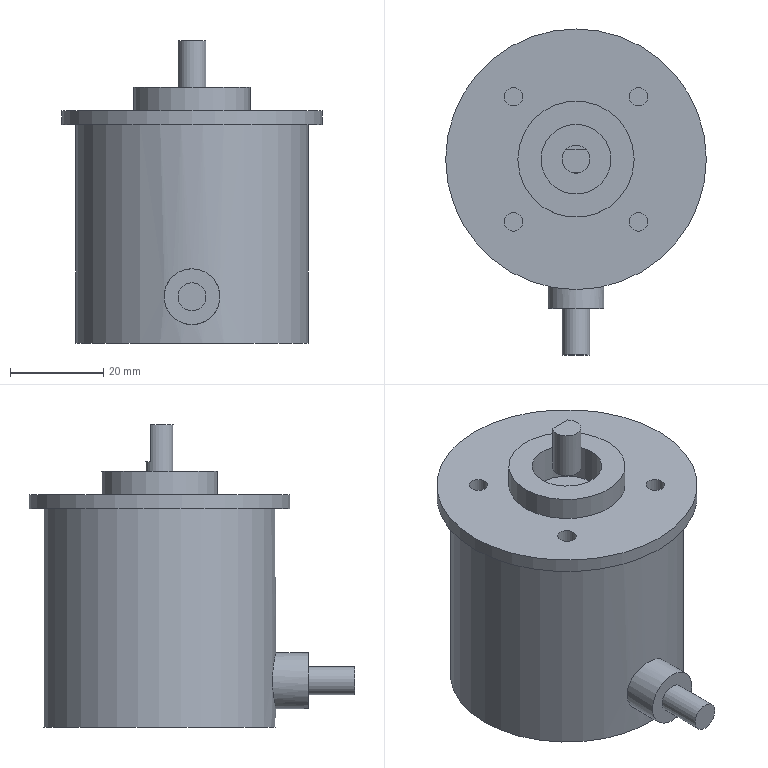Part | NX | features BREP 2 | 2 solids | 26 faces | box 56 x 70 x 65 mm | volume 101579 mm3 | plane 15 | cylinder 11 | commonest cylinder face diameters 4 x4 6 x2 12 x1 15 x1 25 x1 50 x1
STEP:
#1=CARTESIAN_POINT('',(-10.435,-13.435,4.5));
#2=VERTEX_POINT('',#1);
#3=CARTESIAN_POINT('',(-13.435,-13.435,4.5));
#4=DIRECTION('',(0.,0.,-1.));
#5=DIRECTION('',(1.,0.,0.));
#6=AXIS2_PLACEMENT_3D('',#3,#4,#5);
#7=CIRCLE('',#6,3.);
#8=EDGE_CURVE('',#2,#2,#7,.T.);
#9=ORIENTED_EDGE('',*,*,#8,.F.);
#10=EDGE_LOOP('',(#9));
#11=FACE_BOUND('',#10,.T.);
#12=CARTESIAN_POINT('',(-11.199,-11.435,15.));
#13=VERTEX_POINT('',#12);
#14=CARTESIAN_POINT('',(-15.671,-11.435,15.));
#15=VERTEX_POINT('',#14);
#16=CARTESIAN_POINT('',(-13.435,-13.435,15.));
#17=DIRECTION('',(0.,0.,-1.));
#18=DIRECTION('',(1.,0.,0.));
#19=AXIS2_PLACEMENT_3D('',#16,#17,#18);
#20=CIRCLE('',#19,3.);
#21=EDGE_CURVE('',#13,#15,#20,.T.);
#22=ORIENTED_EDGE('',*,*,#21,.T.);
#23=CARTESIAN_POINT('',(-15.671,-11.435,7.));
#24=VERTEX_POINT('',#23);
#25=CARTESIAN_POINT('',(-15.671,-11.435,7.));
#26=DIRECTION('',(0.,0.,-1.));
#27=VECTOR('',#26,1000.);
#28=LINE('',#25,#27);
#29=EDGE_CURVE('',#15,#24,#28,.T.);
#30=ORIENTED_EDGE('',*,*,#29,.T.);
#31=CARTESIAN_POINT('',(-11.199,-11.435,7.));
#32=VERTEX_POINT('',#31);
#33=CARTESIAN_POINT('',(-13.435,-13.435,7.));
#34=DIRECTION('',(0.,0.,1.));
#35=DIRECTION('',(1.,0.,0.));
#36=AXIS2_PLACEMENT_3D('',#33,#34,#35);
#37=CIRCLE('',#36,3.);
#38=EDGE_CURVE('',#32,#24,#37,.T.);
#39=ORIENTED_EDGE('',*,*,#38,.F.);
#40=CARTESIAN_POINT('',(-11.199,-11.435,7.));
#41=DIRECTION('',(0.,0.,-1.));
#42=VECTOR('',#41,1000.);
#43=LINE('',#40,#42);
#44=EDGE_CURVE('',#13,#32,#43,.T.);
#45=ORIENTED_EDGE('',*,*,#44,.F.);
#46=EDGE_LOOP('',(#22,#30,#39,#45));
#47=FACE_BOUND('',#46,.T.);
#48=CARTESIAN_POINT('',(-13.435,-13.435,15.));
#49=DIRECTION('',(0.,0.,-1.));
#50=DIRECTION('',(-1.,0.,0.));
#51=AXIS2_PLACEMENT_3D('',#48,#49,#50);
#52=CYLINDRICAL_SURFACE('',#51,3.);
#53=ADVANCED_FACE('',(#11,#47),#52,.T.);
#54=CARTESIAN_POINT('',(-15.671,-11.435,15.));
#55=DIRECTION('',(1.,0.,0.));
#56=VECTOR('',#55,1000.);
#57=LINE('',#54,#56);
#58=EDGE_CURVE('',#15,#13,#57,.T.);
#59=ORIENTED_EDGE('',*,*,#58,.F.);
#60=ORIENTED_EDGE('',*,*,#21,.F.);
#61=EDGE_LOOP('',(#59,#60));
#62=FACE_BOUND('',#61,.T.);
#63=CARTESIAN_POINT('',(-13.435,-13.435,15.));
#64=DIRECTION('',(0.,0.,1.));
#65=DIRECTION('',(1.,0.,0.));
#66=AXIS2_PLACEMENT_3D('',#63,#64,#65);
#67=PLANE('',#66);
#68=ADVANCED_FACE('',(#62),#67,.T.);
#69=ORIENTED_EDGE('',*,*,#8,.T.);
#70=EDGE_LOOP('',(#69));
#71=FACE_BOUND('',#70,.T.);
#72=CARTESIAN_POINT('',(-13.435,-13.435,4.5));
#73=DIRECTION('',(0.,0.,1.));
#74=DIRECTION('',(1.,0.,0.));
#75=AXIS2_PLACEMENT_3D('',#72,#73,#74);
#76=PLANE('',#75);
#77=ADVANCED_FACE('',(#71),#76,.F.);
#78=ORIENTED_EDGE('',*,*,#58,.T.);
#79=ORIENTED_EDGE('',*,*,#44,.T.);
#80=CARTESIAN_POINT('',(-15.671,-11.435,7.));
#81=DIRECTION('',(1.,0.,0.));
#82=VECTOR('',#81,1000.);
#83=LINE('',#80,#82);
#84=EDGE_CURVE('',#24,#32,#83,.T.);
#85=ORIENTED_EDGE('',*,*,#84,.F.);
#86=ORIENTED_EDGE('',*,*,#29,.F.);
#87=EDGE_LOOP('',(#78,#79,#85,#86));
#88=FACE_BOUND('',#87,.T.);
#89=CARTESIAN_POINT('',(-15.671,-11.435,7.));
#90=DIRECTION('',(0.,-1.,0.));
#91=DIRECTION('',(0.,0.,-1.));
#92=AXIS2_PLACEMENT_3D('',#89,#90,#91);
#93=PLANE('',#92);
#94=ADVANCED_FACE('',(#88),#93,.F.);
#95=ORIENTED_EDGE('',*,*,#38,.T.);
#96=ORIENTED_EDGE('',*,*,#84,.T.);
#97=EDGE_LOOP('',(#95,#96));
#98=FACE_BOUND('',#97,.T.);
#99=CARTESIAN_POINT('',(-13.435,-13.435,7.));
#100=DIRECTION('',(0.,0.,1.));
#101=DIRECTION('',(1.,0.,0.));
#102=AXIS2_PLACEMENT_3D('',#99,#100,#101);
#103=PLANE('',#102);
#104=ADVANCED_FACE('',(#98),#103,.T.);
#105=CLOSED_SHELL('',(#53,#68,#77,#94,#104));
#106=MANIFOLD_SOLID_BREP('',#105);
#107=CARTESIAN_POINT('',(2.,0.,0.));
#108=VERTEX_POINT('',#107);
#109=CARTESIAN_POINT('',(0.,0.,0.));
#110=DIRECTION('',(0.,0.,1.));
#111=DIRECTION('',(1.,0.,0.));
#112=AXIS2_PLACEMENT_3D('',#109,#110,#111);
#113=CIRCLE('',#112,2.);
#114=EDGE_CURVE('',#108,#108,#113,.T.);
#115=ORIENTED_EDGE('',*,*,#114,.T.);
#116=EDGE_LOOP('',(#115));
#117=FACE_BOUND('',#116,.T.);
#118=CARTESIAN_POINT('',(2.,0.,-10.));
#119=VERTEX_POINT('',#118);
#120=CARTESIAN_POINT('',(0.,0.,-10.));
#121=DIRECTION('',(0.,0.,1.));
#122=DIRECTION('',(1.,0.,0.));
#123=AXIS2_PLACEMENT_3D('',#120,#121,#122);
#124=CIRCLE('',#123,2.);
#125=EDGE_CURVE('',#119,#119,#124,.T.);
#126=ORIENTED_EDGE('',*,*,#125,.F.);
#127=EDGE_LOOP('',(#126));
#128=FACE_BOUND('',#127,.T.);
#129=CARTESIAN_POINT('',(0.,0.,0.));
#130=DIRECTION('',(0.,0.,1.));
#131=DIRECTION('',(1.,0.,0.));
#132=AXIS2_PLACEMENT_3D('',#129,#130,#131);
#133=CYLINDRICAL_SURFACE('',#132,2.);
#134=ADVANCED_FACE('',(#117,#128),#133,.F.);
#135=CARTESIAN_POINT('',(-24.87,0.,0.));
#136=VERTEX_POINT('',#135);
#137=CARTESIAN_POINT('',(-26.87,0.,0.));
#138=DIRECTION('',(0.,0.,1.));
#139=DIRECTION('',(1.,0.,0.));
#140=AXIS2_PLACEMENT_3D('',#137,#138,#139);
#141=CIRCLE('',#140,2.);
#142=EDGE_CURVE('',#136,#136,#141,.T.);
#143=ORIENTED_EDGE('',*,*,#142,.T.);
#144=EDGE_LOOP('',(#143));
#145=FACE_BOUND('',#144,.T.);
#146=CARTESIAN_POINT('',(-24.87,0.,-10.));
#147=VERTEX_POINT('',#146);
#148=CARTESIAN_POINT('',(-26.87,0.,-10.));
#149=DIRECTION('',(0.,0.,1.));
#150=DIRECTION('',(1.,0.,0.));
#151=AXIS2_PLACEMENT_3D('',#148,#149,#150);
#152=CIRCLE('',#151,2.);
#153=EDGE_CURVE('',#147,#147,#152,.T.);
#154=ORIENTED_EDGE('',*,*,#153,.F.);
#155=EDGE_LOOP('',(#154));
#156=FACE_BOUND('',#155,.T.);
#157=CARTESIAN_POINT('',(-26.87,0.,0.));
#158=DIRECTION('',(0.,0.,1.));
#159=DIRECTION('',(1.,0.,0.));
#160=AXIS2_PLACEMENT_3D('',#157,#158,#159);
#161=CYLINDRICAL_SURFACE('',#160,2.);
#162=ADVANCED_FACE('',(#145,#156),#161,.F.);
#163=CARTESIAN_POINT('',(-24.87,-26.87,0.));
#164=VERTEX_POINT('',#163);
#165=CARTESIAN_POINT('',(-26.87,-26.87,0.));
#166=DIRECTION('',(0.,0.,1.));
#167=DIRECTION('',(1.,0.,0.));
#168=AXIS2_PLACEMENT_3D('',#165,#166,#167);
#169=CIRCLE('',#168,2.);
#170=EDGE_CURVE('',#164,#164,#169,.T.);
#171=ORIENTED_EDGE('',*,*,#170,.T.);
#172=EDGE_LOOP('',(#171));
#173=FACE_BOUND('',#172,.T.);
#174=CARTESIAN_POINT('',(-24.87,-26.87,-10.));
#175=VERTEX_POINT('',#174);
#176=CARTESIAN_POINT('',(-26.87,-26.87,-10.));
#177=DIRECTION('',(0.,0.,1.));
#178=DIRECTION('',(1.,0.,0.));
#179=AXIS2_PLACEMENT_3D('',#176,#177,#178);
#180=CIRCLE('',#179,2.);
#181=EDGE_CURVE('',#175,#175,#180,.T.);
#182=ORIENTED_EDGE('',*,*,#181,.F.);
#183=EDGE_LOOP('',(#182));
#184=FACE_BOUND('',#183,.T.);
#185=CARTESIAN_POINT('',(-26.87,-26.87,0.));
#186=DIRECTION('',(0.,0.,1.));
#187=DIRECTION('',(1.,0.,0.));
#188=AXIS2_PLACEMENT_3D('',#185,#186,#187);
#189=CYLINDRICAL_SURFACE('',#188,2.);
#190=ADVANCED_FACE('',(#173,#184),#189,.F.);
#191=CARTESIAN_POINT('',(2.,-26.87,0.));
#192=VERTEX_POINT('',#191);
#193=CARTESIAN_POINT('',(0.,-26.87,0.));
#194=DIRECTION('',(0.,0.,1.));
#195=DIRECTION('',(1.,0.,0.));
#196=AXIS2_PLACEMENT_3D('',#193,#194,#195);
#197=CIRCLE('',#196,2.);
#198=EDGE_CURVE('',#192,#192,#197,.T.);
#199=ORIENTED_EDGE('',*,*,#198,.T.);
#200=EDGE_LOOP('',(#199));
#201=FACE_BOUND('',#200,.T.);
#202=CARTESIAN_POINT('',(2.,-26.87,-10.));
#203=VERTEX_POINT('',#202);
#204=CARTESIAN_POINT('',(0.,-26.87,-10.));
#205=DIRECTION('',(0.,0.,1.));
#206=DIRECTION('',(1.,0.,0.));
#207=AXIS2_PLACEMENT_3D('',#204,#205,#206);
#208=CIRCLE('',#207,2.);
#209=EDGE_CURVE('',#203,#203,#208,.T.);
#210=ORIENTED_EDGE('',*,*,#209,.F.);
#211=EDGE_LOOP('',(#210));
#212=FACE_BOUND('',#211,.T.);
#213=CARTESIAN_POINT('',(0.,-26.87,0.));
#214=DIRECTION('',(0.,0.,1.));
#215=DIRECTION('',(1.,0.,0.));
#216=AXIS2_PLACEMENT_3D('',#213,#214,#215);
#217=CYLINDRICAL_SURFACE('',#216,2.);
#218=ADVANCED_FACE('',(#201,#212),#217,.F.);
#219=CARTESIAN_POINT('',(-13.435,-55.435,-43.));
#220=VERTEX_POINT('',#219);
#221=CARTESIAN_POINT('',(-13.435,-55.435,-40.));
#222=DIRECTION('',(0.,-1.,0.));
#223=DIRECTION('',(0.,0.,-1.));
#224=AXIS2_PLACEMENT_3D('',#221,#222,#223);
#225=CIRCLE('',#224,3.);
#226=EDGE_CURVE('',#220,#220,#225,.T.);
#227=ORIENTED_EDGE('',*,*,#226,.F.);
#228=EDGE_LOOP('',(#227));
#229=FACE_BOUND('',#228,.T.);
#230=CARTESIAN_POINT('',(-13.435,-45.435,-43.));
#231=VERTEX_POINT('',#230);
#232=CARTESIAN_POINT('',(-13.435,-45.435,-40.));
#233=DIRECTION('',(0.,-1.,0.));
#234=DIRECTION('',(0.,0.,-1.));
#235=AXIS2_PLACEMENT_3D('',#232,#233,#234);
#236=CIRCLE('',#235,3.);
#237=EDGE_CURVE('',#231,#231,#236,.T.);
#238=ORIENTED_EDGE('',*,*,#237,.T.);
#239=EDGE_LOOP('',(#238));
#240=FACE_BOUND('',#239,.T.);
#241=CARTESIAN_POINT('',(-13.435,-37.704,-40.));
#242=DIRECTION('',(0.,-1.,0.));
#243=DIRECTION('',(0.,0.,-1.));
#244=AXIS2_PLACEMENT_3D('',#241,#242,#243);
#245=CYLINDRICAL_SURFACE('',#244,3.);
#246=ADVANCED_FACE('',(#229,#240),#245,.T.);
#247=CARTESIAN_POINT('',(-13.435,-45.435,-46.));
#248=VERTEX_POINT('',#247);
#249=CARTESIAN_POINT('',(-13.435,-45.435,-40.));
#250=DIRECTION('',(0.,-1.,0.));
#251=DIRECTION('',(0.,0.,-1.));
#252=AXIS2_PLACEMENT_3D('',#249,#250,#251);
#253=CIRCLE('',#252,6.);
#254=EDGE_CURVE('',#248,#248,#253,.T.);
#255=ORIENTED_EDGE('',*,*,#254,.F.);
#256=EDGE_LOOP('',(#255));
#257=FACE_BOUND('',#256,.T.);
#258=CARTESIAN_POINT('',(-13.435,-38.435,-34.));
#259=VERTEX_POINT('',#258);
#260=CARTESIAN_POINT('',(-18.141,-38.074,-35.302));
#261=CARTESIAN_POINT('',(-13.434,-38.615,-33.349));
#262=CARTESIAN_POINT('',(-8.732,-38.075,-35.302));
#263=CARTESIAN_POINT('',(-6.786,-37.519,-39.993));
#264=CARTESIAN_POINT('',(-8.733,-38.075,-44.703));
#265=CARTESIAN_POINT('',(-13.432,-38.615,-46.648));
#266=CARTESIAN_POINT('',(-18.133,-38.076,-44.706));
#267=CARTESIAN_POINT('',(-20.084,-37.519,-40.003));
#268=CARTESIAN_POINT('',(-18.141,-38.074,-35.302));
#269=CARTESIAN_POINT('',(-13.434,-38.615,-33.349));
#270=CARTESIAN_POINT('',(-8.732,-38.075,-35.302));
#271=B_SPLINE_CURVE_WITH_KNOTS('',3,(#260,#261,#262,#263,#264,#265,#266,#267,#268,#269,#270),.UNSPECIFIED.,.T.,.F.,(1,1,1,1,1,1,1,1,1,1,1,1,1,1,1),(-0.01412,-0.009413,-0.004706,0.,0.004706,0.009413,0.01412,0.01883,0.02353,0.02824,0.03294,0.03765,0.04236,0.04706,0.05177),.UNSPECIFIED.);
#272=EDGE_CURVE('',#259,#259,#271,.T.);
#273=ORIENTED_EDGE('',*,*,#272,.F.);
#274=EDGE_LOOP('',(#273));
#275=FACE_BOUND('',#274,.T.);
#276=CARTESIAN_POINT('',(-13.435,-37.704,-40.));
#277=DIRECTION('',(0.,-1.,0.));
#278=DIRECTION('',(0.,0.,-1.));
#279=AXIS2_PLACEMENT_3D('',#276,#277,#278);
#280=CYLINDRICAL_SURFACE('',#279,6.);
#281=ADVANCED_FACE('',(#257,#275),#280,.T.);
#282=CARTESIAN_POINT('',(-38.435,-13.435,-3.));
#283=VERTEX_POINT('',#282);
#284=CARTESIAN_POINT('',(-13.435,-13.435,-3.));
#285=DIRECTION('',(0.,0.,-1.));
#286=DIRECTION('',(-1.,0.,0.));
#287=AXIS2_PLACEMENT_3D('',#284,#285,#286);
#288=CIRCLE('',#287,25.);
#289=EDGE_CURVE('',#283,#283,#288,.T.);
#290=ORIENTED_EDGE('',*,*,#289,.T.);
#291=EDGE_LOOP('',(#290));
#292=FACE_BOUND('',#291,.T.);
#293=CARTESIAN_POINT('',(-38.435,-13.435,-50.));
#294=VERTEX_POINT('',#293);
#295=CARTESIAN_POINT('',(-13.435,-13.435,-50.));
#296=DIRECTION('',(0.,0.,-1.));
#297=DIRECTION('',(-1.,0.,0.));
#298=AXIS2_PLACEMENT_3D('',#295,#296,#297);
#299=CIRCLE('',#298,25.);
#300=EDGE_CURVE('',#294,#294,#299,.T.);
#301=ORIENTED_EDGE('',*,*,#300,.F.);
#302=EDGE_LOOP('',(#301));
#303=FACE_BOUND('',#302,.T.);
#304=ORIENTED_EDGE('',*,*,#272,.T.);
#305=EDGE_LOOP('',(#304));
#306=FACE_BOUND('',#305,.T.);
#307=CARTESIAN_POINT('',(-13.435,-13.435,-50.));
#308=DIRECTION('',(0.,0.,1.));
#309=DIRECTION('',(1.,0.,0.));
#310=AXIS2_PLACEMENT_3D('',#307,#308,#309);
#311=CYLINDRICAL_SURFACE('',#310,25.);
#312=ADVANCED_FACE('',(#292,#303,#306),#311,.T.);
#313=CARTESIAN_POINT('',(-5.935,-13.435,5.));
#314=VERTEX_POINT('',#313);
#315=CARTESIAN_POINT('',(-13.435,-13.435,5.));
#316=DIRECTION('',(0.,0.,1.));
#317=DIRECTION('',(1.,0.,0.));
#318=AXIS2_PLACEMENT_3D('',#315,#316,#317);
#319=CIRCLE('',#318,7.5);
#320=EDGE_CURVE('',#314,#314,#319,.T.);
#321=ORIENTED_EDGE('',*,*,#320,.T.);
#322=EDGE_LOOP('',(#321));
#323=FACE_BOUND('',#322,.T.);
#324=CARTESIAN_POINT('',(-5.935,-13.435,-3.));
#325=VERTEX_POINT('',#324);
#326=CARTESIAN_POINT('',(-13.435,-13.435,-3.));
#327=DIRECTION('',(0.,0.,1.));
#328=DIRECTION('',(1.,0.,0.));
#329=AXIS2_PLACEMENT_3D('',#326,#327,#328);
#330=CIRCLE('',#329,7.5);
#331=EDGE_CURVE('',#325,#325,#330,.T.);
#332=ORIENTED_EDGE('',*,*,#331,.F.);
#333=EDGE_LOOP('',(#332));
#334=FACE_BOUND('',#333,.T.);
#335=CARTESIAN_POINT('',(-13.435,-13.435,5.));
#336=DIRECTION('',(0.,0.,1.));
#337=DIRECTION('',(1.,0.,0.));
#338=AXIS2_PLACEMENT_3D('',#335,#336,#337);
#339=CYLINDRICAL_SURFACE('',#338,7.5);
#340=ADVANCED_FACE('',(#323,#334),#339,.F.);
#341=CARTESIAN_POINT('',(-0.935,-13.435,0.));
#342=VERTEX_POINT('',#341);
#343=CARTESIAN_POINT('',(-13.435,-13.435,0.));
#344=DIRECTION('',(0.,0.,1.));
#345=DIRECTION('',(1.,0.,0.));
#346=AXIS2_PLACEMENT_3D('',#343,#344,#345);
#347=CIRCLE('',#346,12.5);
#348=EDGE_CURVE('',#342,#342,#347,.T.);
#349=ORIENTED_EDGE('',*,*,#348,.T.);
#350=EDGE_LOOP('',(#349));
#351=FACE_BOUND('',#350,.T.);
#352=CARTESIAN_POINT('',(-0.935,-13.435,5.));
#353=VERTEX_POINT('',#352);
#354=CARTESIAN_POINT('',(-13.435,-13.435,5.));
#355=DIRECTION('',(0.,0.,1.));
#356=DIRECTION('',(1.,0.,0.));
#357=AXIS2_PLACEMENT_3D('',#354,#355,#356);
#358=CIRCLE('',#357,12.5);
#359=EDGE_CURVE('',#353,#353,#358,.T.);
#360=ORIENTED_EDGE('',*,*,#359,.F.);
#361=EDGE_LOOP('',(#360));
#362=FACE_BOUND('',#361,.T.);
#363=CARTESIAN_POINT('',(-13.435,-13.435,5.));
#364=DIRECTION('',(0.,0.,-1.));
#365=DIRECTION('',(-1.,0.,0.));
#366=AXIS2_PLACEMENT_3D('',#363,#364,#365);
#367=CYLINDRICAL_SURFACE('',#366,12.5);
#368=ADVANCED_FACE('',(#351,#362),#367,.T.);
#369=CARTESIAN_POINT('',(14.565,-13.435,0.));
#370=VERTEX_POINT('',#369);
#371=CARTESIAN_POINT('',(-13.435,-13.435,0.));
#372=DIRECTION('',(0.,0.,1.));
#373=DIRECTION('',(1.,0.,0.));
#374=AXIS2_PLACEMENT_3D('',#371,#372,#373);
#375=CIRCLE('',#374,28.);
#376=EDGE_CURVE('',#370,#370,#375,.T.);
#377=ORIENTED_EDGE('',*,*,#376,.F.);
#378=EDGE_LOOP('',(#377));
#379=FACE_BOUND('',#378,.T.);
#380=CARTESIAN_POINT('',(14.565,-13.435,-3.));
#381=VERTEX_POINT('',#380);
#382=CARTESIAN_POINT('',(-13.435,-13.435,-3.));
#383=DIRECTION('',(0.,0.,1.));
#384=DIRECTION('',(1.,0.,0.));
#385=AXIS2_PLACEMENT_3D('',#382,#383,#384);
#386=CIRCLE('',#385,28.);
#387=EDGE_CURVE('',#381,#381,#386,.T.);
#388=ORIENTED_EDGE('',*,*,#387,.T.);
#389=EDGE_LOOP('',(#388));
#390=FACE_BOUND('',#389,.T.);
#391=CARTESIAN_POINT('',(-13.435,-13.435,-3.));
#392=DIRECTION('',(0.,0.,1.));
#393=DIRECTION('',(1.,0.,0.));
#394=AXIS2_PLACEMENT_3D('',#391,#392,#393);
#395=CYLINDRICAL_SURFACE('',#394,28.);
#396=ADVANCED_FACE('',(#379,#390),#395,.T.);
#397=ORIENTED_EDGE('',*,*,#387,.F.);
#398=EDGE_LOOP('',(#397));
#399=FACE_BOUND('',#398,.T.);
#400=ORIENTED_EDGE('',*,*,#289,.F.);
#401=EDGE_LOOP('',(#400));
#402=FACE_BOUND('',#401,.T.);
#403=CARTESIAN_POINT('',(14.565,-13.435,-3.));
#404=DIRECTION('',(0.,0.,-1.));
#405=DIRECTION('',(-1.,0.,0.));
#406=AXIS2_PLACEMENT_3D('',#403,#404,#405);
#407=PLANE('',#406);
#408=ADVANCED_FACE('',(#399,#402),#407,.T.);
#409=ORIENTED_EDGE('',*,*,#114,.F.);
#410=EDGE_LOOP('',(#409));
#411=FACE_BOUND('',#410,.T.);
#412=ORIENTED_EDGE('',*,*,#142,.F.);
#413=EDGE_LOOP('',(#412));
#414=FACE_BOUND('',#413,.T.);
#415=ORIENTED_EDGE('',*,*,#170,.F.);
#416=EDGE_LOOP('',(#415));
#417=FACE_BOUND('',#416,.T.);
#418=ORIENTED_EDGE('',*,*,#198,.F.);
#419=EDGE_LOOP('',(#418));
#420=FACE_BOUND('',#419,.T.);
#421=ORIENTED_EDGE('',*,*,#376,.T.);
#422=EDGE_LOOP('',(#421));
#423=FACE_BOUND('',#422,.T.);
#424=ORIENTED_EDGE('',*,*,#348,.F.);
#425=EDGE_LOOP('',(#424));
#426=FACE_BOUND('',#425,.T.);
#427=CARTESIAN_POINT('',(-13.435,-13.435,0.));
#428=DIRECTION('',(0.,0.,1.));
#429=DIRECTION('',(1.,0.,0.));
#430=AXIS2_PLACEMENT_3D('',#427,#428,#429);
#431=PLANE('',#430);
#432=ADVANCED_FACE('',(#411,#414,#417,#420,#423,#426),#431,.T.);
#433=ORIENTED_EDGE('',*,*,#320,.F.);
#434=EDGE_LOOP('',(#433));
#435=FACE_BOUND('',#434,.T.);
#436=ORIENTED_EDGE('',*,*,#359,.T.);
#437=EDGE_LOOP('',(#436));
#438=FACE_BOUND('',#437,.T.);
#439=CARTESIAN_POINT('',(-13.435,-13.435,5.));
#440=DIRECTION('',(0.,0.,1.));
#441=DIRECTION('',(1.,0.,0.));
#442=AXIS2_PLACEMENT_3D('',#439,#440,#441);
#443=PLANE('',#442);
#444=ADVANCED_FACE('',(#435,#438),#443,.T.);
#445=ORIENTED_EDGE('',*,*,#331,.T.);
#446=EDGE_LOOP('',(#445));
#447=FACE_BOUND('',#446,.T.);
#448=CARTESIAN_POINT('',(-13.435,-13.435,-3.));
#449=DIRECTION('',(0.,0.,-1.));
#450=DIRECTION('',(-1.,0.,0.));
#451=AXIS2_PLACEMENT_3D('',#448,#449,#450);
#452=PLANE('',#451);
#453=ADVANCED_FACE('',(#447),#452,.F.);
#454=ORIENTED_EDGE('',*,*,#300,.T.);
#455=EDGE_LOOP('',(#454));
#456=FACE_BOUND('',#455,.T.);
#457=CARTESIAN_POINT('',(-13.435,-13.435,-50.));
#458=DIRECTION('',(0.,0.,-1.));
#459=DIRECTION('',(-1.,0.,0.));
#460=AXIS2_PLACEMENT_3D('',#457,#458,#459);
#461=PLANE('',#460);
#462=ADVANCED_FACE('',(#456),#461,.T.);
#463=ORIENTED_EDGE('',*,*,#226,.T.);
#464=EDGE_LOOP('',(#463));
#465=FACE_BOUND('',#464,.T.);
#466=CARTESIAN_POINT('',(-13.435,-55.435,-40.));
#467=DIRECTION('',(0.,-1.,0.));
#468=DIRECTION('',(0.,0.,-1.));
#469=AXIS2_PLACEMENT_3D('',#466,#467,#468);
#470=PLANE('',#469);
#471=ADVANCED_FACE('',(#465),#470,.T.);
#472=ORIENTED_EDGE('',*,*,#254,.T.);
#473=EDGE_LOOP('',(#472));
#474=FACE_BOUND('',#473,.T.);
#475=ORIENTED_EDGE('',*,*,#237,.F.);
#476=EDGE_LOOP('',(#475));
#477=FACE_BOUND('',#476,.T.);
#478=CARTESIAN_POINT('',(-13.435,-45.435,-43.));
#479=DIRECTION('',(0.,-1.,0.));
#480=DIRECTION('',(0.,0.,-1.));
#481=AXIS2_PLACEMENT_3D('',#478,#479,#480);
#482=PLANE('',#481);
#483=ADVANCED_FACE('',(#474,#477),#482,.T.);
#484=ORIENTED_EDGE('',*,*,#209,.T.);
#485=EDGE_LOOP('',(#484));
#486=FACE_BOUND('',#485,.T.);
#487=CARTESIAN_POINT('',(0.,-26.87,-10.));
#488=DIRECTION('',(0.,0.,-1.));
#489=DIRECTION('',(-1.,0.,0.));
#490=AXIS2_PLACEMENT_3D('',#487,#488,#489);
#491=PLANE('',#490);
#492=ADVANCED_FACE('',(#486),#491,.F.);
#493=ORIENTED_EDGE('',*,*,#181,.T.);
#494=EDGE_LOOP('',(#493));
#495=FACE_BOUND('',#494,.T.);
#496=CARTESIAN_POINT('',(-26.87,-26.87,-10.));
#497=DIRECTION('',(0.,0.,-1.));
#498=DIRECTION('',(-1.,0.,0.));
#499=AXIS2_PLACEMENT_3D('',#496,#497,#498);
#500=PLANE('',#499);
#501=ADVANCED_FACE('',(#495),#500,.F.);
#502=ORIENTED_EDGE('',*,*,#153,.T.);
#503=EDGE_LOOP('',(#502));
#504=FACE_BOUND('',#503,.T.);
#505=CARTESIAN_POINT('',(-26.87,0.,-10.));
#506=DIRECTION('',(0.,0.,-1.));
#507=DIRECTION('',(-1.,0.,0.));
#508=AXIS2_PLACEMENT_3D('',#505,#506,#507);
#509=PLANE('',#508);
#510=ADVANCED_FACE('',(#504),#509,.F.);
#511=ORIENTED_EDGE('',*,*,#125,.T.);
#512=EDGE_LOOP('',(#511));
#513=FACE_BOUND('',#512,.T.);
#514=CARTESIAN_POINT('',(0.,0.,-10.));
#515=DIRECTION('',(0.,0.,-1.));
#516=DIRECTION('',(-1.,0.,0.));
#517=AXIS2_PLACEMENT_3D('',#514,#515,#516);
#518=PLANE('',#517);
#519=ADVANCED_FACE('',(#513),#518,.F.);
#520=CLOSED_SHELL('',(#134,#162,#190,#218,#246,#281,#312,#340,#368,#396,#408,#432,#444,#453,#462,#471,#483,#492,#501,#510,#519));
#521=MANIFOLD_SOLID_BREP('',#520);
#522=(LENGTH_UNIT()NAMED_UNIT(*)SI_UNIT(.MILLI.,.METRE.));
#523=UNCERTAINTY_MEASURE_WITH_UNIT(LENGTH_MEASURE(0.0508),#522,'','');
#524=(NAMED_UNIT(*)PLANE_ANGLE_UNIT()SI_UNIT($,.RADIAN.));
#525=(NAMED_UNIT(*)SI_UNIT($,.STERADIAN.)SOLID_ANGLE_UNIT());
#526=(GEOMETRIC_REPRESENTATION_CONTEXT(3)GLOBAL_UNCERTAINTY_ASSIGNED_CONTEXT((#523))GLOBAL_UNIT_ASSIGNED_CONTEXT((#522,#524,#525))REPRESENTATION_CONTEXT('',''));
#527=ADVANCED_BREP_SHAPE_REPRESENTATION('',(#106,#521),#526);